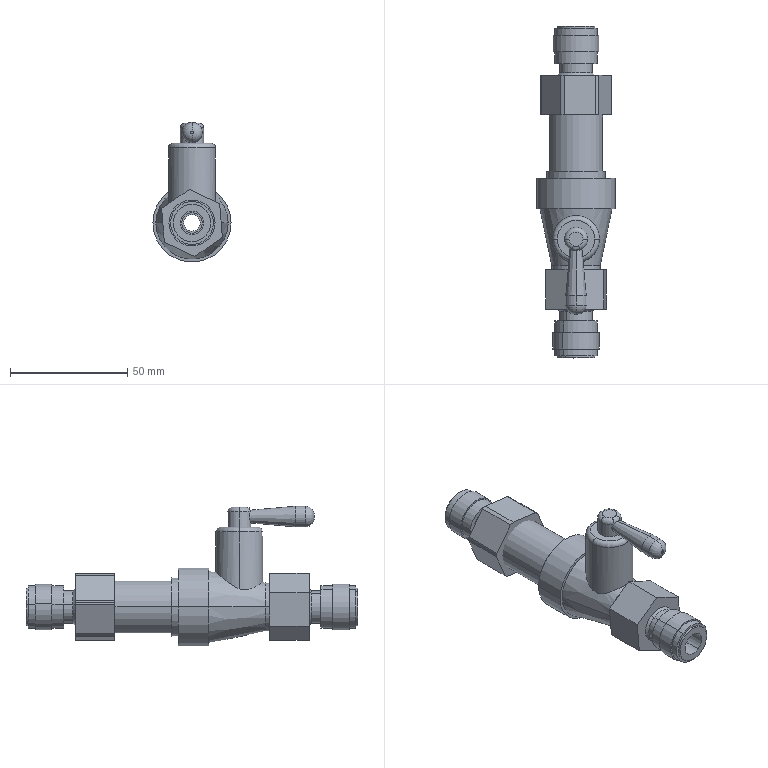Part | SolidWorks | features BaseBody 3 | 3 solids | 111 faces | box 33.3 x 141.4 x 59.55 mm | volume 62869 mm3 | cylinder 55 | plane 38 | cone 10 | torus 7 | spline 1 | commonest cylinder face diameters 30 x7 10 x4 14 x4 16 x4 18.2 x4 18.3 x4